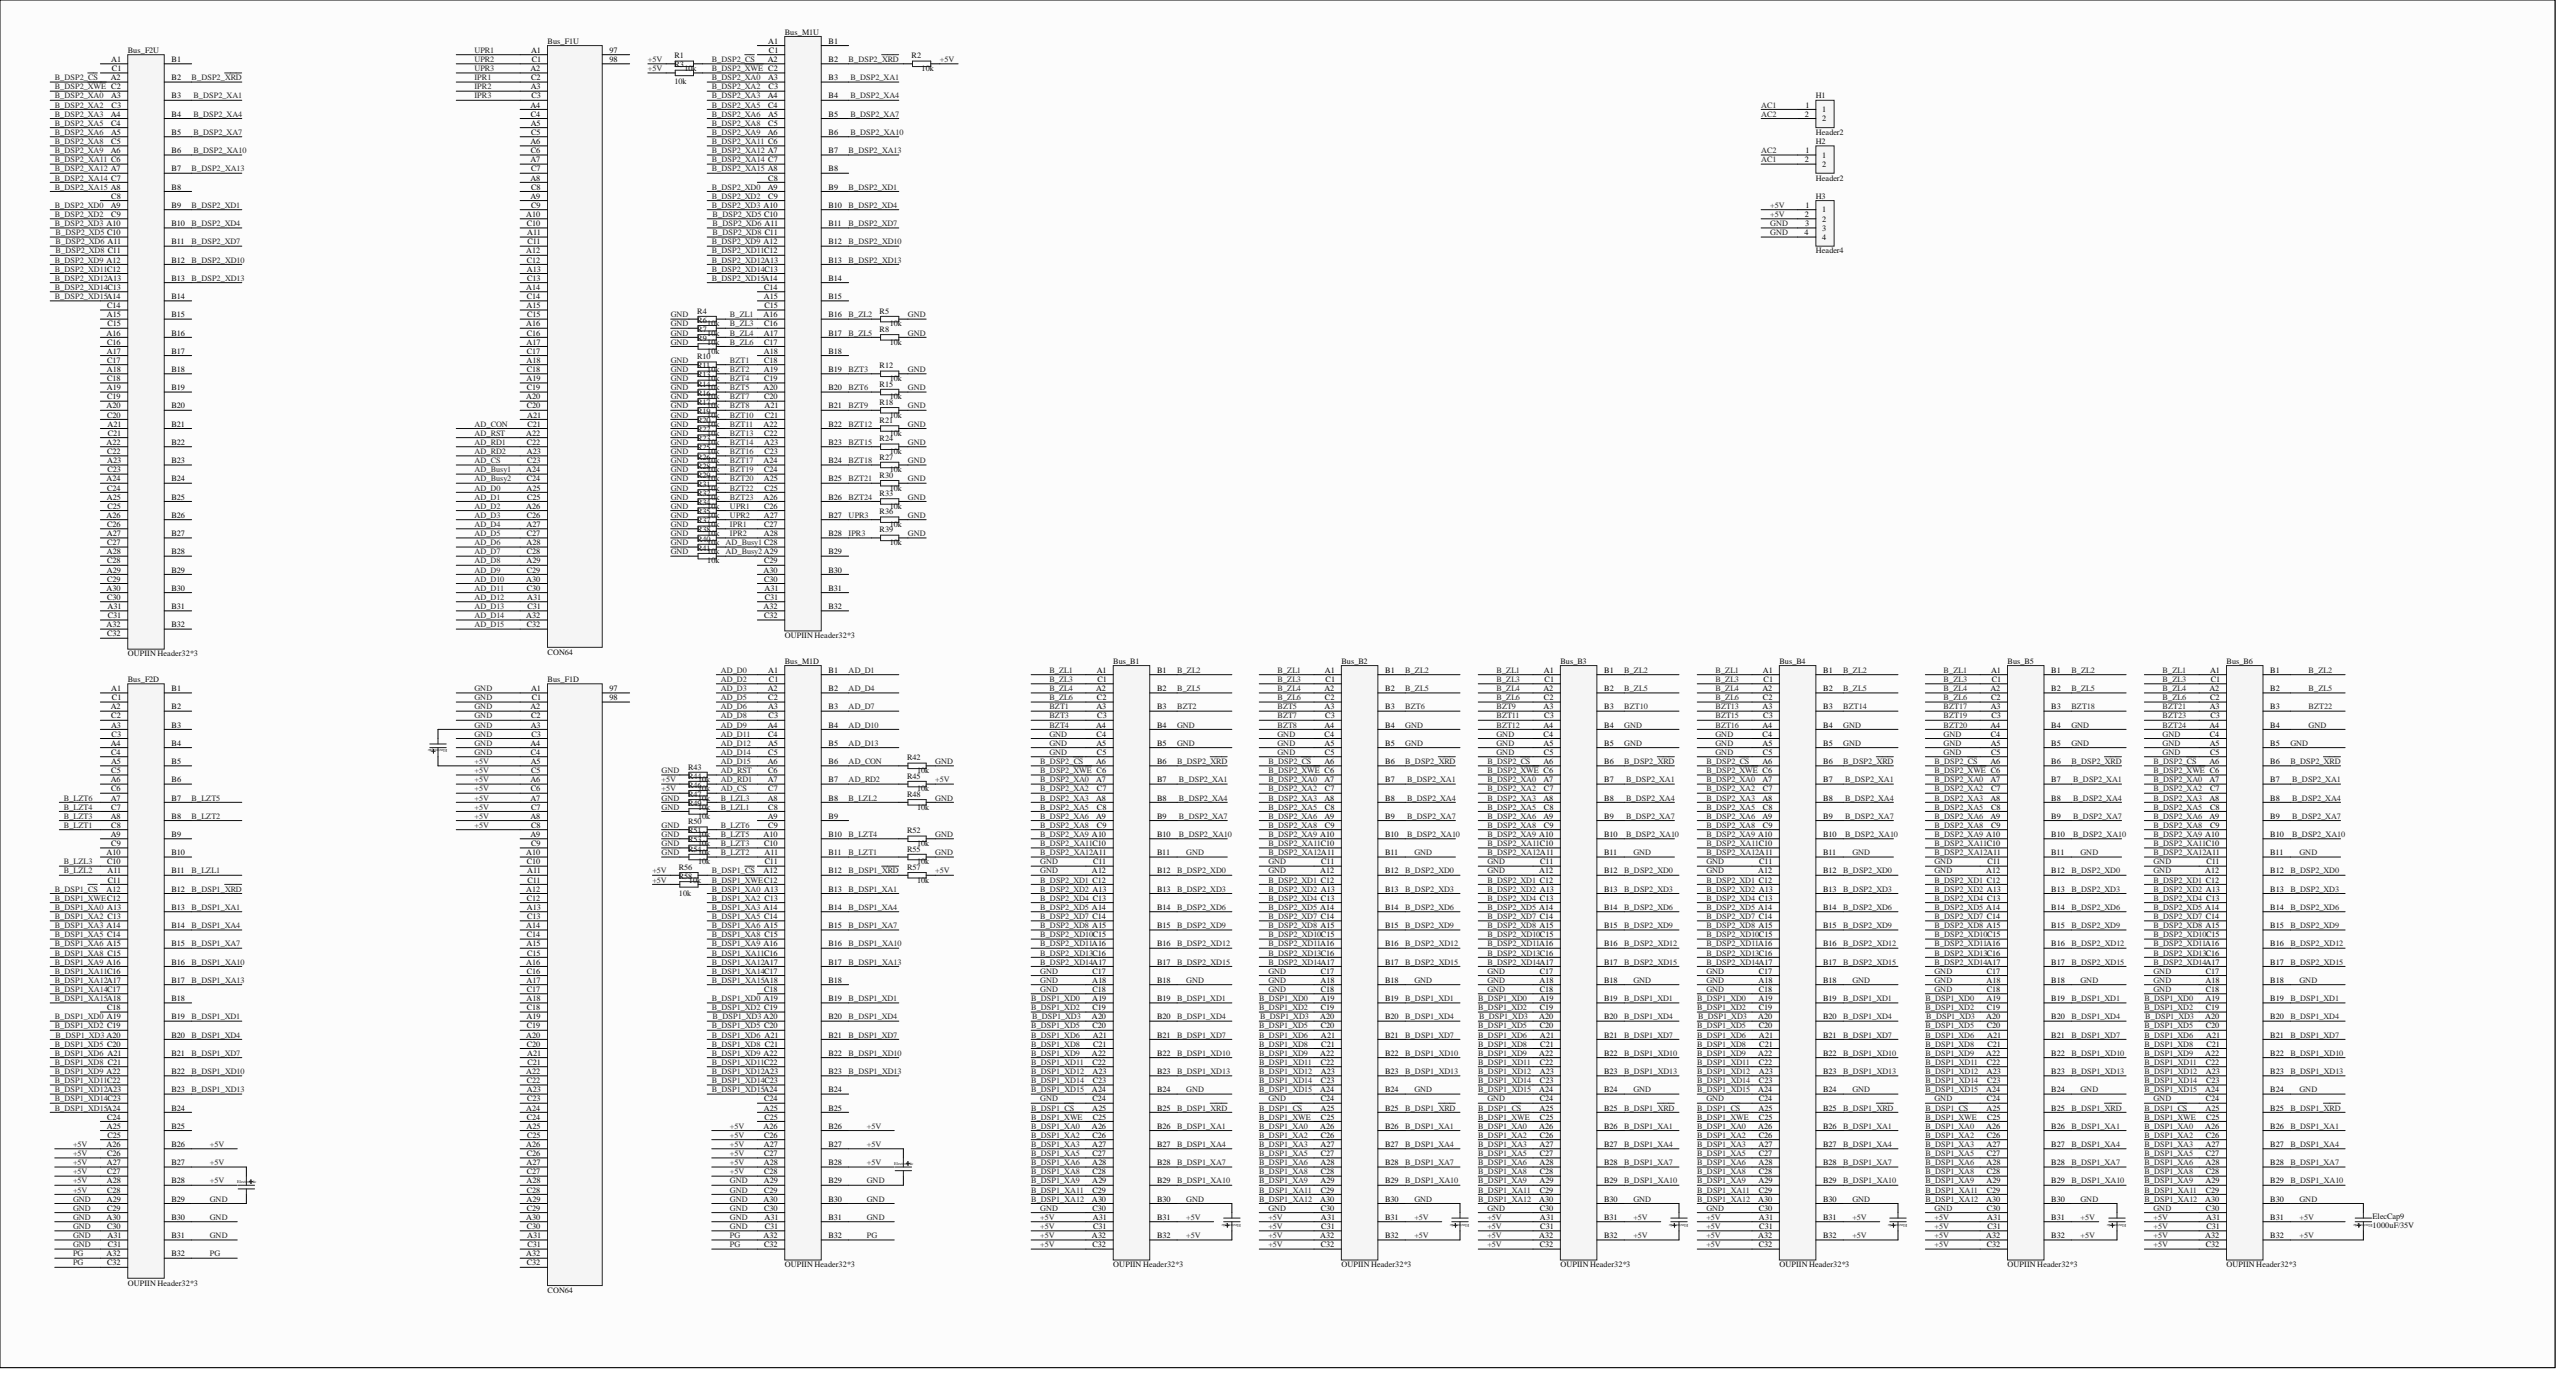Circuit board | Altium Designer | 82 parts | 143 nets
Bill of materials:
Comment,Description,Designator,Footprint,LibRef,Quantity
"OUPIIN Header32*3","OUPIIN Header32*3","Bus_B1, Bus_B2, Bus_B3, Bus_B4, Bus_B5, Bus_B6, Bus_F2D, Bus_F2U, Bus_M1D, Bus_M1U","OUPIINBus32*3_zhili","OUPIIN Header32*3","10"
"CON64","Euro-style pin header 64-pos","Bus_F1D, Bus_F1U","OUPIINBus32*2_zhili","CON64","2"
"1000uF/35V","Electrolytic Capacitor(Pin1 Positive)","ElecCap1, ElecCap2, ElecCap3, ElecCap4, ElecCap5, ElecCap6, ElecCap7, ElecCap8, ElecCap9","1000UF/35V","ELECTROCap","9"
"Header2","Header2","H1","EDGCon_2p_5.08mm","Header2","1"
"Header2","Header2","H2","EDGCON_2p_5.08mm_ear","Header2","1"
"Header4","Header4","H3","EDGCON_4p_5.08mm","Header4","1"
"10k","","R1, R2, R3, R4, R5, R6, R7, R8, R9, R10, R11, R12, R13, R14, R15, R16, R17, R18, R19, R20, R21, R22, R23, R24, R25, R26, R27, R28, R29, R30, R31, R32, R33, R34, R35, R36, R37, R38, R39, R40, R41, R42, R43, R44, R45, R46, R47, R48, R49, R50, R51, R52, R53, R54, R55, R56, R57, R58","0603","RES2","58"
Netlist (Protel format):
[
Bus_B1
OUPIINBus32*3_zhili
OUPIIN Header32*3



]
[
Bus_B2
OUPIINBus32*3_zhili
OUPIIN Header32*3



]
[
Bus_B3
OUPIINBus32*3_zhili
OUPIIN Header32*3



]
[
Bus_B4
OUPIINBus32*3_zhili
OUPIIN Header32*3



]
[
Bus_B5
OUPIINBus32*3_zhili
OUPIIN Header32*3



]
[
Bus_B6
OUPIINBus32*3_zhili
OUPIIN Header32*3



]
[
Bus_F1D
OUPIINBus32*2_zhili
CON64



]
[
Bus_F1U
OUPIINBus32*2_zhili
CON64



]
[
Bus_F2D
OUPIINBus32*3_zhili
OUPIIN Header32*3



]
[
Bus_F2U
OUPIINBus32*3_zhili
OUPIIN Header32*3



]
[
Bus_M1D
OUPIINBus32*3_zhili
OUPIIN Header32*3



]
[
Bus_M1U
OUPIINBus32*3_zhili
OUPIIN Header32*3



]
[
ElecCap1
1000UF/35V
1000uF/35V



]
[
ElecCap2
1000UF/35V
1000uF/35V



]
[
ElecCap3
1000UF/35V
1000uF/35V



]
[
ElecCap4
1000UF/35V
1000uF/35V



]
[
ElecCap5
1000UF/35V
1000uF/35V



]
[
ElecCap6
1000UF/35V
1000uF/35V



]
[
ElecCap7
1000UF/35V
1000uF/35V



]
[
ElecCap8
1000UF/35V
1000uF/35V



]
[
ElecCap9
1000UF/35V
1000uF/35V



]
[
H1
EDGCon_2p_5.08mm
Header2



]
[
H2
EDGCON_2p_5.08mm_ear
Header2



]
[
H3
EDGCON_4p_5.08mm
Header4



]
[
R1
0603
10k



]
[
R2
0603
10k



]
[
R3
0603
10k



]
[
R4
0603
10k



]
[
R5
0603
10k



]
[
R6
0603
10k



]
[
R7
0603
10k



]
[
R8
0603
10k



]
[
R9
0603
10k



]
[
R10
0603
10k



]
[
R11
0603
10k



]
[
R12
0603
10k



]
[
R13
0603
10k



]
[
R14
0603
10k



]
[
R15
0603
10k



]
[
R16
0603
10k



]
[
R17
0603
10k



]
[
R18
0603
10k



]
[
R19
0603
10k



]
[
R20
0603
10k



]
[
R21
0603
10k



]
[
R22
0603
10k



]
[
R23
0603
10k



]
[
R24
0603
10k



]
[
R25
0603
10k



]
[
R26
0603
10k



]
[
R27
0603
10k



]
[
R28
0603
10k



]
[
R29
0603
10k



]
[
R30
0603
10k



]
[
R31
0603
10k



]
[
R32
0603
10k



]
[
R33
0603
10k



]
[
R34
0603
10k



]
[
R35
0603
10k



]
[
R36
0603
10k



]
[
R37
0603
10k



]
[
R38
0603
10k



]
[
R39
0603
10k



]
[
R40
0603
10k



]
[
R41
0603
10k



]
[
R42
0603
10k



]
[
R43
0603
10k



]
[
R44
0603
10k



]
[
R45
0603
10k



]
[
R46
0603
10k



]
[
R47
0603
10k



]
[
R48
0603
10k



]
[
R49
0603
10k



]
[
R50
0603
10k



]
[
R51
0603
10k



]
[
R52
0603
10k



]
[
R53
0603
10k



]
[
R54
0603
10k



]
[
R55
0603
10k



]
[
R56
0603
10k



]
[
R57
0603
10k



]
[
R58
0603
10k



]
(
UPR3
Bus_F1U-A2
Bus_M1U-B27
R36-1
)
(
UPR2
Bus_F1U-C1
Bus_M1U-A27
R35-2
)
(
UPR1
Bus_F1U-A1
Bus_M1U-C26
R34-2
)
(
PG
Bus_F2D-A32
Bus_F2D-B32
Bus_F2D-C32
Bus_M1D-A32
Bus_M1D-B32
Bus_M1D-C32
)
(
IPR3
Bus_F1U-C3
Bus_M1U-B28
R39-1
)
(
IPR2
Bus_F1U-A3
Bus_M1U-A28
R38-2
)
(
IPR1
Bus_F1U-C2
Bus_M1U-C27
R37-2
)
(
GND
Bus_B1-A5
Bus_B1-A12
Bus_B1-A18
Bus_B1-B4
Bus_B1-B5
Bus_B1-B11
Bus_B1-B18
Bus_B1-B24
Bus_B1-B30
Bus_B1-C4
Bus_B1-C5
Bus_B1-C11
Bus_B1-C17
Bus_B1-C18
Bus_B1-C24
Bus_B1-C30
Bus_B2-A5
Bus_B2-A12
Bus_B2-A18
Bus_B2-B4
Bus_B2-B5
Bus_B2-B11
Bus_B2-B18
Bus_B2-B24
Bus_B2-B30
Bus_B2-C4
Bus_B2-C5
Bus_B2-C11
Bus_B2-C17
Bus_B2-C18
Bus_B2-C24
Bus_B2-C30
Bus_B3-A5
Bus_B3-A12
Bus_B3-A18
Bus_B3-B4
Bus_B3-B5
Bus_B3-B11
Bus_B3-B18
Bus_B3-B24
Bus_B3-B30
Bus_B3-C4
Bus_B3-C5
Bus_B3-C11
Bus_B3-C17
Bus_B3-C18
Bus_B3-C24
Bus_B3-C30
Bus_B4-A5
Bus_B4-A12
Bus_B4-A18
Bus_B4-B4
Bus_B4-B5
Bus_B4-B11
Bus_B4-B18
Bus_B4-B24
Bus_B4-B30
Bus_B4-C4
Bus_B4-C5
Bus_B4-C11
Bus_B4-C17
Bus_B4-C18
Bus_B4-C24
Bus_B4-C30
Bus_B5-A5
Bus_B5-A12
Bus_B5-A18
Bus_B5-B4
Bus_B5-B5
Bus_B5-B11
Bus_B5-B18
Bus_B5-B24
Bus_B5-B30
Bus_B5-C4
Bus_B5-C5
Bus_B5-C11
Bus_B5-C17
Bus_B5-C18
Bus_B5-C24
Bus_B5-C30
Bus_B6-A5
Bus_B6-A12
Bus_B6-A18
Bus_B6-B4
Bus_B6-B5
Bus_B6-B11
Bus_B6-B18
Bus_B6-B24
Bus_B6-B30
Bus_B6-C4
Bus_B6-C5
Bus_B6-C11
Bus_B6-C17
Bus_B6-C18
Bus_B6-C24
Bus_B6-C30
Bus_F1D-A1
Bus_F1D-A2
Bus_F1D-A3
Bus_F1D-A4
Bus_F1D-C1
Bus_F1D-C2
Bus_F1D-C3
Bus_F1D-C4
Bus_F2D-A29
Bus_F2D-A30
Bus_F2D-A31
Bus_F2D-B29
Bus_F2D-B30
Bus_F2D-B31
Bus_F2D-C29
Bus_F2D-C30
Bus_F2D-C31
Bus_M1D-A29
Bus_M1D-A30
Bus_M1D-A31
Bus_M1D-B29
Bus_M1D-B30
Bus_M1D-B31
Bus_M1D-C29
Bus_M1D-C30
Bus_M1D-C31
ElecCap1-2
ElecCap2-2
ElecCap3-2
ElecCap4-2
ElecCap5-2
ElecCap6-2
ElecCap7-2
ElecCap8-2
ElecCap9-2
H3-3
H3-4
R4-1
R5-2
R6-1
R7-1
R8-2
R9-1
R10-1
R11-1
R12-2
R13-1
R14-1
R15-2
R16-1
R17-1
R18-2
R19-1
R20-1
R21-2
R22-1
R23-1
R24-2
R25-1
R26-1
R27-2
R28-1
R29-1
R30-2
R31-1
R32-1
R33-2
R34-1
R35-1
R36-2
R37-1
R38-1
R39-2
R40-1
R41-1
R42-2
R43-1
R47-1
R48-2
R49-1
R50-1
R51-1
R52-2
R53-1
R54-1
R55-2
)
(
BZT24
Bus_B6-A4
Bus_M1U-B26
R33-1
)
(
BZT23
Bus_B6-C3
Bus_M1U-A26
R32-2
)
(
BZT22
Bus_B6-B3
Bus_M1U-C25
R31-2
)
(
BZT21
Bus_B6-A3
Bus_M1U-B25
R30-1
)
(
BZT20
Bus_B5-A4
Bus_M1U-A25
R29-2
)
(
BZT19
Bus_B5-C3
Bus_M1U-C24
R28-2
)
(
BZT18
Bus_B5-B3
Bus_M1U-B24
R27-1
)
(
BZT17
Bus_B5-A3
Bus_M1U-A24
R26-2
)
(
BZT16
Bus_B4-A4
Bus_M1U-C23
R25-2
)
(
BZT15
Bus_B4-C3
Bus_M1U-B23
R24-1
)
(
BZT14
Bus_B4-B3
Bus_M1U-A23
R23-2
)
(
BZT13
Bus_B4-A3
Bus_M1U-C22
R22-2
)
(
BZT12
Bus_B3-A4
Bus_M1U-B22
R21-1
)
(
BZT11
Bus_B3-C3
Bus_M1U-A22
R20-2
)
(
BZT10
Bus_B3-B3
Bus_M1U-C21
R19-2
)
(
BZT9
Bus_B3-A3
Bus_M1U-B21
R18-1
)
(
BZT8
Bus_B2-A4
Bus_M1U-A21
R17-2
)
(
BZT7
Bus_B2-C3
Bus_M1U-C20
R16-2
)
(
BZT6
Bus_B2-B3
Bus_M1U-B20
R15-1
)
(
BZT5
Bus_B2-A3
Bus_M1U-A20
R14-2
)
(
BZT4
Bus_B1-A4
Bus_M1U-C19
R13-2
)
(
BZT3
Bus_B1-C3
Bus_M1U-B19
R12-1
)
(
BZT2
Bus_B1-B3
Bus_M1U-A19
R11-2
)
(
BZT1
Bus_B1-A3
Bus_M1U-C18
R10-2
)
(
B_ZL6
Bus_B1-C2
Bus_B2-C2
Bus_B3-C2
Bus_B4-C2
Bus_B5-C2
Bus_B6-C2
Bus_M1U-C17
R9-2
)
(
B_ZL5
Bus_B1-B2
Bus_B2-B2
Bus_B3-B2
Bus_B4-B2
Bus_B5-B2
Bus_B6-B2
Bus_M1U-B17
R8-1
)
(
B_ZL4
Bus_B1-A2
Bus_B2-A2
Bus_B3-A2
Bus_B4-A2
Bus_B5-A2
Bus_B6-A2
Bus_M1U-A17
R7-2
)
(
B_ZL3
Bus_B1-C1
Bus_B2-C1
Bus_B3-C1
Bus_B4-C1
Bus_B5-C1
Bus_B6-C1
Bus_M1U-C16
R6-2
)
(
B_ZL2
Bus_B1-B1
Bus_B2-B1
Bus_B3-B1
Bus_B4-B1
Bus_B5-B1
Bus_B6-B1
Bus_M1U-B16
R5-1
)
(
B_ZL1
Bus_B1-A1
Bus_B2-A1
Bus_B3-A1
Bus_B4-A1
Bus_B5-A1
Bus_B6-A1
Bus_M1U-A16
R4-2
)
(
B_LZT6
Bus_F2D-A7
Bus_M1D-C9
R50-2
)
(
B_LZT5
Bus_F2D-B7
Bus_M1D-A10
R51-2
)
(
B_LZT4
Bus_F2D-C7
Bus_M1D-B10
R52-1
)
(
B_LZT3
Bus_F2D-A8
Bus_M1D-C10
R53-2
)
(
B_LZT2
Bus_F2D-B8
Bus_M1D-A11
R54-2
)
(
B_LZT1
Bus_F2D-C8
Bus_M1D-B11
R55-1
)
(
B_LZL3
Bus_F2D-C10
Bus_M1D-A8
R47-2
)
(
B_LZL2
Bus_F2D-A11
Bus_M1D-B8
R48-1
)
(
B_LZL1
Bus_F2D-B11
Bus_M1D-C8
R49-2
)
(
B_DSP2_XD15
Bus_B1-B17
Bus_B2-B17
Bus_B3-B17
Bus_B4-B17
Bus_B5-B17
Bus_B6-B17
Bus_F2U-A14
Bus_M1U-A14
)
(
B_DSP2_XD14
Bus_B1-A17
Bus_B2-A17
Bus_B3-A17
Bus_B4-A17
Bus_B5-A17
Bus_B6-A17
Bus_F2U-C13
Bus_M1U-C13
)
(
B_DSP2_XD13
Bus_B1-C16
Bus_B2-C16
Bus_B3-C16
Bus_B4-C16
Bus_B5-C16
Bus_B6-C16
Bus_F2U-B13
Bus_M1U-B13
)
(
B_DSP2_XD12
Bus_B1-B16
Bus_B2-B16
Bus_B3-B16
Bus_B4-B16
Bus_B5-B16
Bus_B6-B16
Bus_F2U-A13
Bus_M1U-A13
)
(
B_DSP2_XD11
Bus_B1-A16
Bus_B2-A16
Bus_B3-A16
Bus_B4-A16
Bus_B5-A16
Bus_B6-A16
Bus_F2U-C12
Bus_M1U-C12
)
(
B_DSP2_XD10
Bus_B1-C15
Bus_B2-C15
Bus_B3-C15
Bus_B4-C15
Bus_B5-C15
Bus_B6-C15
Bus_F2U-B12
Bus_M1U-B12
)
(
B_DSP2_XD9
Bus_B1-B15
Bus_B2-B15
Bus_B3-B15
Bus_B4-B15
Bus_B5-B15
Bus_B6-B15
Bus_F2U-A12
Bus_M1U-A12
)
(
B_DSP2_XD8
Bus_B1-A15
Bus_B2-A15
Bus_B3-A15
Bus_B4-A15
Bus_B5-A15
Bus_B6-A15
Bus_F2U-C11
Bus_M1U-C11
)
(
B_DSP2_XD7
Bus_B1-C14
Bus_B2-C14
Bus_B3-C14
Bus_B4-C14
Bus_B5-C14
Bus_B6-C14
Bus_F2U-B11
Bus_M1U-B11
)
(
B_DSP2_XD6
Bus_B1-B14
Bus_B2-B14
Bus_B3-B14
Bus_B4-B14
Bus_B5-B14
Bus_B6-B14
Bus_F2U-A11
Bus_M1U-A11
)
(
B_DSP2_XD5
Bus_B1-A14
Bus_B2-A14
Bus_B3-A14
Bus_B4-A14
Bus_B5-A14
Bus_B6-A14
Bus_F2U-C10
Bus_M1U-C10
)
(
B_DSP2_XD4
Bus_B1-C13
Bus_B2-C13
Bus_B3-C13
Bus_B4-C13
Bus_B5-C13
Bus_B6-C13
Bus_F2U-B10
Bus_M1U-B10
)
(
B_DSP2_XD3
Bus_B1-B13
Bus_B2-B13
Bus_B3-B13
Bus_B4-B13
Bus_B5-B13
Bus_B6-B13
Bus_F2U-A10
Bus_M1U-A10
)
(
B_DSP2_XD2
Bus_B1-A13
Bus_B2-A13
Bus_B3-A13
Bus_B4-A13
Bus_B5-A13
Bus_B6-A13
Bus_F2U-C9
Bus_M1U-C9
)
(
B_DSP2_XD1
Bus_B1-C12
Bus_B2-C12
Bus_B3-C12
Bus_B4-C12
Bus_B5-C12
Bus_B6-C12
Bus_F2U-B9
Bus_M1U-B9
)
(
B_DSP2_XD0
Bus_B1-B12
Bus_B2-B12
Bus_B3-B12
Bus_B4-B12
Bus_B5-B12
Bus_B6-B12
Bus_F2U-A9
Bus_M1U-A9
)
(
B_DSP2_XA15
Bus_F2U-A8
Bus_M1U-A8
)
(
B_DSP2_XA14
Bus_F2U-C7
Bus_M1U-C7
)
(
B_DSP2_XA13
Bus_F2U-B7
Bus_M1U-B7
)
(
B_DSP2_XA12
Bus_B1-A11
Bus_B2-A11
Bus_B3-A11
Bus_B4-A11
Bus_B5-A11
Bus_B6-A11
Bus_F2U-A7
Bus_M1U-A7
)
(
B_DSP2_XA11
Bus_B1-C10
Bus_B2-C10
Bus_B3-C10
Bus_B4-C10
Bus_B5-C10
Bus_B6-C10
Bus_F2U-C6
Bus_M1U-C6
)
(
B_DSP2_XA10
Bus_B1-B10
Bus_B2-B10
Bus_B3-B10
Bus_B4-B10
Bus_B5-B10
Bus_B6-B10
Bus_F2U-B6
Bus_M1U-B6
)
(
B_DSP2_XA9
Bus_B1-A10
Bus_B2-A10
Bus_B3-A10
Bus_B4-A10
Bus_B5-A10
Bus_B6-A10
Bus_F2U-A6
Bus_M1U-A6
)
(
B_DSP2_XA8
Bus_B1-C9
Bus_B2-C9
Bus_B3-C9
Bus_B4-C9
Bus_B5-C9
Bus_B6-C9
Bus_F2U-C5
Bus_M1U-C5
)
(
B_DSP2_XA7
Bus_B1-B9
Bus_B2-B9
Bus_B3-B9
Bus_B4-B9
Bus_B5-B9
Bus_B6-B9
Bus_F2U-B5
Bus_M1U-B5
)
(
B_DSP2_XA6
Bus_B1-A9
Bus_B2-A9
Bus_B3-A9
Bus_B4-A9
Bus_B5-A9
Bus_B6-A9
Bus_F2U-A5
Bus_M1U-A5
)
(
B_DSP2_XA5
Bus_B1-C8
Bus_B2-C8
Bus_B3-C8
Bus_B4-C8
Bus_B5-C8
Bus_B6-C8
Bus_F2U-C4
Bus_M1U-C4
)
(
B_DSP2_XA4
Bus_B1-B8
Bus_B2-B8
Bus_B3-B8
Bus_B4-B8
Bus_B5-B8
Bus_B6-B8
Bus_F2U-B4
Bus_M1U-B4
)
(
B_DSP2_XA3
Bus_B1-A8
Bus_B2-A8
Bus_B3-A8
Bus_B4-A8
Bus_B5-A8
Bus_B6-A8
Bus_F2U-A4
Bus_M1U-A4
)
(
B_DSP2_XA2
Bus_B1-C7
Bus_B2-C7
Bus_B3-C7
Bus_B4-C7
Bus_B5-C7
Bus_B6-C7
Bus_F2U-C3
Bus_M1U-C3
)
(
B_DSP2_XA1
Bus_B1-B7
Bus_B2-B7
Bus_B3-B7
Bus_B4-B7
Bus_B5-B7
Bus_B6-B7
Bus_F2U-B3
Bus_M1U-B3
)
(
B_DSP2_XA0
Bus_B1-A7
Bus_B2-A7
Bus_B3-A7
Bus_B4-A7
Bus_B5-A7
Bus_B6-A7
Bus_F2U-A3
Bus_M1U-A3
)
(
B_DSP2_X\W\E\
Bus_B1-C6
Bus_B2-C6
Bus_B3-C6
Bus_B4-C6
Bus_B5-C6
Bus_B6-C6
Bus_F2U-C2
Bus_M1U-C2
R3-2
)
(
B_DSP2_X\R\D\
Bus_B1-B6
Bus_B2-B6
Bus_B3-B6
Bus_B4-B6
Bus_B5-B6
Bus_B6-B6
Bus_F2U-B2
Bus_M1U-B2
R2-1
)
(
B_DSP2_C\S\
Bus_B1-A6
Bus_B2-A6
Bus_B3-A6
Bus_B4-A6
Bus_B5-A6
Bus_B6-A6
Bus_F2U-A2
Bus_M1U-A2
R1-2
)
(
B_DSP1_XD15
Bus_B1-A24
Bus_B2-A24
Bus_B3-A24
Bus_B4-A24
Bus_B5-A24
Bus_B6-A24
Bus_F2D-A24
Bus_M1D-A24
)
(
B_DSP1_XD14
Bus_B1-C23
Bus_B2-C23
Bus_B3-C23
Bus_B4-C23
Bus_B5-C23
Bus_B6-C23
Bus_F2D-C23
Bus_M1D-C23
)
(
B_DSP1_XD13
Bus_B1-B23
Bus_B2-B23
Bus_B3-B23
Bus_B4-B23
Bus_B5-B23
Bus_B6-B23
Bus_F2D-B23
Bus_M1D-B23
)
(
B_DSP1_XD12
Bus_B1-A23
Bus_B2-A23
Bus_B3-A23
Bus_B4-A23
Bus_B5-A23
Bus_B6-A23
Bus_F2D-A23
Bus_M1D-A23
)
(
B_DSP1_XD11
Bus_B1-C22
Bus_B2-C22
Bus_B3-C22
Bus_B4-C22
Bus_B5-C22
Bus_B6-C22
Bus_F2D-C22
Bus_M1D-C22
)
(
B_DSP1_XD10
Bus_B1-B22
Bus_B2-B22
Bus_B3-B22
Bus_B4-B22
Bus_B5-B22
Bus_B6-B22
Bus_F2D-B22
Bus_M1D-B22
)
(
B_DSP1_XD9
Bus_B1-A22
Bus_B2-A22
Bus_B3-A22
Bus_B4-A22
Bus_B5-A22
Bus_B6-A22
Bus_F2D-A22
Bus_M1D-A22
)
(
B_DSP1_XD8
Bus_B1-C21
Bus_B2-C21
Bus_B3-C21
Bus_B4-C21
Bus_B5-C21
Bus_B6-C21
Bus_F2D-C21
Bus_M1D-C21
)
(
B_DSP1_XD7
Bus_B1-B21
Bus_B2-B21
Bus_B3-B21
Bus_B4-B21
Bus_B5-B21
Bus_B6-B21
Bus_F2D-B21
Bus_M1D-B21
)
(
B_DSP1_XD6
Bus_B1-A21
Bus_B2-A21
Bus_B3-A21
Bus_B4-A21
Bus_B5-A21
Bus_B6-A21
Bus_F2D-A21
Bus_M1D-A21
)
(
B_DSP1_XD5
Bus_B1-C20
Bus_B2-C20
Bus_B3-C20
Bus_B4-C20
Bus_B5-C20
Bus_B6-C20
Bus_F2D-C20
Bus_M1D-C20
)
(
B_DSP1_XD4
Bus_B1-B20
Bus_B2-B20
Bus_B3-B20
Bus_B4-B20
Bus_B5-B20
Bus_B6-B20
Bus_F2D-B20
Bus_M1D-B20
)
(
B_DSP1_XD3
Bus_B1-A20
Bus_B2-A20
Bus_B3-A20
Bus_B4-A20
Bus_B5-A20
Bus_B6-A20
Bus_F2D-A20
Bus_M1D-A20
)
(
B_DSP1_XD2
Bus_B1-C19
Bus_B2-C19
Bus_B3-C19
Bus_B4-C19
Bus_B5-C19
Bus_B6-C19
Bus_F2D-C19
Bus_M1D-C19
)
(
B_DSP1_XD1
Bus_B1-B19
Bus_B2-B19
Bus_B3-B19
Bus_B4-B19
Bus_B5-B19
Bus_B6-B19
Bus_F2D-B19
Bus_M1D-B19
)
(
B_DSP1_XD0
Bus_B1-A19
Bus_B2-A19
Bus_B3-A19
Bus_B4-A19
Bus_B5-A19
Bus_B6-A19
Bus_F2D-A19
Bus_M1D-A19
)
(
B_DSP1_XA15
Bus_F2D-A18
Bus_M1D-A18
)
(
B_DSP1_XA14
Bus_F2D-C17
Bus_M1D-C17
)
(
B_DSP1_XA13
Bus_F2D-B17
Bus_M1D-B17
)
(
B_DSP1_XA12
Bus_B1-A30
Bus_B2-A30
Bus_B3-A30
Bus_B4-A30
Bus_B5-A30
Bus_B6-A30
Bus_F2D-A17
Bus_M1D-A17
)
(
B_DSP1_XA11
Bus_B1-C29
Bus_B2-C29
Bus_B3-C29
Bus_B4-C29
Bus_B5-C29
Bus_B6-C29
Bus_F2D-C16
Bus_M1D-C16
)
(
B_DSP1_XA10
Bus_B1-B29
Bus_B2-B29
Bus_B3-B29
Bus_B4-B29
Bus_B5-B29
Bus_B6-B29
Bus_F2D-B16
Bus_M1D-B16
)
(
B_DSP1_XA9
Bus_B1-A29
Bus_B2-A29
Bus_B3-A29
Bus_B4-A29
Bus_B5-A29
Bus_B6-A29
Bus_F2D-A16
Bus_M1D-A16
)
(
B_DSP1_XA8
Bus_B1-C28
Bus_B2-C28
Bus_B3-C28
Bus_B4-C28
Bus_B5-C28
Bus_B6-C28
Bus_F2D-C15
Bus_M1D-C15
)
(
B_DSP1_XA7
Bus_B1-B28
Bus_B2-B28
Bus_B3-B28
Bus_B4-B28
Bus_B5-B28
Bus_B6-B28
Bus_F2D-B15
Bus_M1D-B15
)
(
B_DSP1_XA6
Bus_B1-A28
Bus_B2-A28
Bus_B3-A28
Bus_B4-A28
Bus_B5-A28
Bus_B6-A28
Bus_F2D-A15
Bus_M1D-A15
)
(
B_DSP1_XA5
Bus_B1-C27
Bus_B2-C27
Bus_B3-C27
Bus_B4-C27
Bus_B5-C27
Bus_B6-C27
Bus_F2D-C14
Bus_M1D-C14
)
(
B_DSP1_XA4
Bus_B1-B27
Bus_B2-B27
Bus_B3-B27
Bus_B4-B27
Bus_B5-B27
Bus_B6-B27
Bus_F2D-B14
Bus_M1D-B14
)
(
B_DSP1_XA3
Bus_B1-A27
Bus_B2-A27
Bus_B3-A27
Bus_B4-A27
Bus_B5-A27
Bus_B6-A27
Bus_F2D-A14
Bus_M1D-A14
)
(
B_DSP1_XA2
Bus_B1-C26
Bus_B2-C26
Bus_B3-C26
Bus_B4-C26
Bus_B5-C26
Bus_B6-C26
Bus_F2D-C13
Bus_M1D-C13
)
(
B_DSP1_XA1
Bus_B1-B26
Bus_B2-B26
Bus_B3-B26
Bus_B4-B26
Bus_B5-B26
Bus_B6-B26
Bus_F2D-B13
Bus_M1D-B13
)
(
B_DSP1_XA0
Bus_B1-A26
Bus_B2-A26
Bus_B3-A26
Bus_B4-A26
Bus_B5-A26
Bus_B6-A26
Bus_F2D-A13
Bus_M1D-A13
)
(
B_DSP1_X\W\E\
Bus_B1-C25
Bus_B2-C25
Bus_B3-C25
Bus_B4-C25
Bus_B5-C25
Bus_B6-C25
Bus_F2D-C12
Bus_M1D-C12
R58-2
)
(
B_DSP1_X\R\D\
Bus_B1-B25
Bus_B2-B25
Bus_B3-B25
Bus_B4-B25
Bus_B5-B25
Bus_B6-B25
Bus_F2D-B12
Bus_M1D-B12
R57-1
)
(
B_DSP1_C\S\
Bus_B1-A25
Bus_B2-A25
Bus_B3-A25
Bus_B4-A25
Bus_B5-A25
Bus_B6-A25
Bus_F2D-A12
Bus_M1D-A12
R56-2
)
(
AD_RST
Bus_F1U-A22
Bus_M1D-C6
R43-2
)
(
AD_RD2
Bus_F1U-A23
Bus_M1D-B7
R45-1
)
(
AD_RD1
Bus_F1U-C22
Bus_M1D-A7
R44-2
)
(
AD_D15
Bus_F1U-C32
Bus_M1D-A6
)
(
AD_D14
Bus_F1U-A32
Bus_M1D-C5
)
(
AD_D13
Bus_F1U-C31
Bus_M1D-B5
)
(
AD_D12
Bus_F1U-A31
Bus_M1D-A5
)
(
AD_D11
Bus_F1U-C30
Bus_M1D-C4
)
(
AD_D10
Bus_F1U-A30
Bus_M1D-B4
)
(
AD_D9
Bus_F1U-C29
Bus_M1D-A4
)
(
AD_D8
Bus_F1U-A29
Bus_M1D-C3
)
(
AD_D7
Bus_F1U-C28
Bus_M1D-B3
)
(
AD_D6
Bus_F1U-A28
Bus_M1D-A3
)
(
AD_D5
Bus_F1U-C27
Bus_M1D-C2
)
(
AD_D4
Bus_F1U-A27
Bus_M1D-B2
)
(
AD_D3
Bus_F1U-C26
Bus_M1D-A2
)
(
AD_D2
Bus_F1U-A26
Bus_M1D-C1
)
(
AD_D1
Bus_F1U-C25
Bus_M1D-B1
)
(
AD_D0
Bus_F1U-A25
Bus_M1D-A1
)
(
AD_CS
Bus_F1U-C23
Bus_M1D-C7
R46-2
)
(
AD_CON
Bus_F1U-C21
Bus_M1D-B6
R42-1
)
(
AD_Busy2
Bus_F1U-C24
Bus_M1U-A29
R41-2
)
(
AD_Busy1
Bus_F1U-A24
Bus_M1U-C28
R40-2
)
(
AC2
H1-2
H2-1
)
(
AC1
H1-1
H2-2
)
(
+5V
Bus_B1-A31
Bus_B1-A32
Bus_B1-B31
Bus_B1-B32
Bus_B1-C31
Bus_B1-C32
Bus_B2-A31
Bus_B2-A32
Bus_B2-B31
Bus_B2-B32
Bus_B2-C31
Bus_B2-C32
Bus_B3-A31
Bus_B3-A32
Bus_B3-B31
Bus_B3-B32
Bus_B3-C31
Bus_B3-C32
Bus_B4-A31
Bus_B4-A32
Bus_B4-B31
Bus_B4-B32
Bus_B4-C31
Bus_B4-C32
Bus_B5-A31
Bus_B5-A32
Bus_B5-B31
Bus_B5-B32
Bus_B5-C31
Bus_B5-C32
Bus_B6-A31
Bus_B6-A32
Bus_B6-B31
Bus_B6-B32
Bus_B6-C31
Bus_B6-C32
Bus_F1D-A5
Bus_F1D-A6
Bus_F1D-A7
Bus_F1D-A8
Bus_F1D-C5
Bus_F1D-C6
Bus_F1D-C7
Bus_F1D-C8
Bus_F2D-A26
Bus_F2D-A27
Bus_F2D-A28
Bus_F2D-B26
Bus_F2D-B27
Bus_F2D-B28
Bus_F2D-C26
Bus_F2D-C27
Bus_F2D-C28
Bus_M1D-A26
Bus_M1D-A27
Bus_M1D-A28
Bus_M1D-B26
Bus_M1D-B27
Bus_M1D-B28
Bus_M1D-C26
Bus_M1D-C27
Bus_M1D-C28
ElecCap1-1
ElecCap2-1
ElecCap3-1
ElecCap4-1
ElecCap5-1
ElecCap6-1
ElecCap7-1
ElecCap8-1
ElecCap9-1
H3-1
H3-2
R1-1
R2-2
R3-1
R44-1
R45-2
R46-1
R56-1
R57-2
R58-1
)